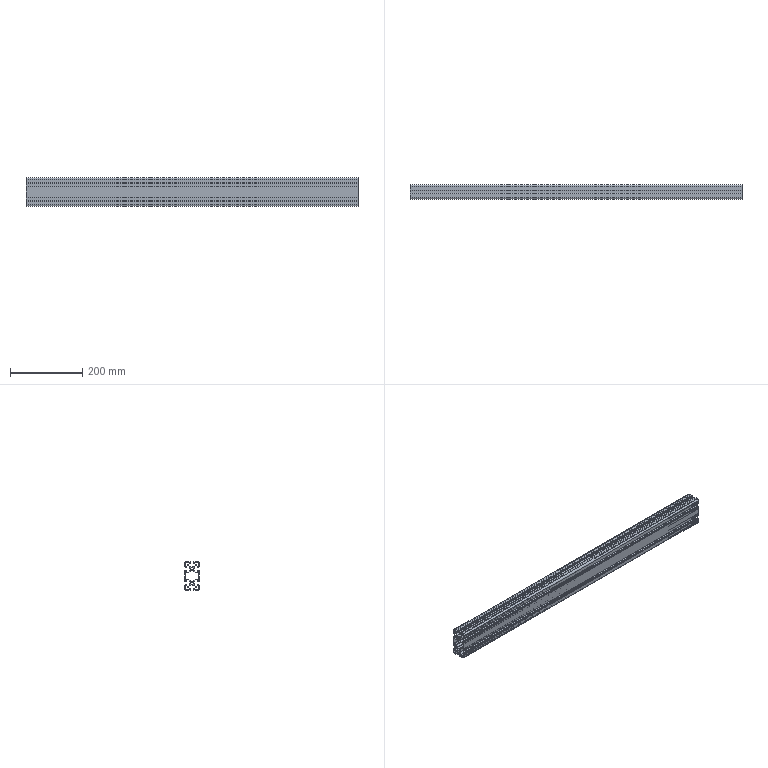Part | STEP file | MK-8-4080H-L-00 Profile 4080H Standard 920mm | 1 solid | 286 faces | box 920 x 40 x 80 mm | volume 746832 mm3 | cylinder 144 | plane 142 | commonest cylinder face diameters 0.6 x44 2 x44 4 x28 0.4 x14 6 x4 6.8 x4